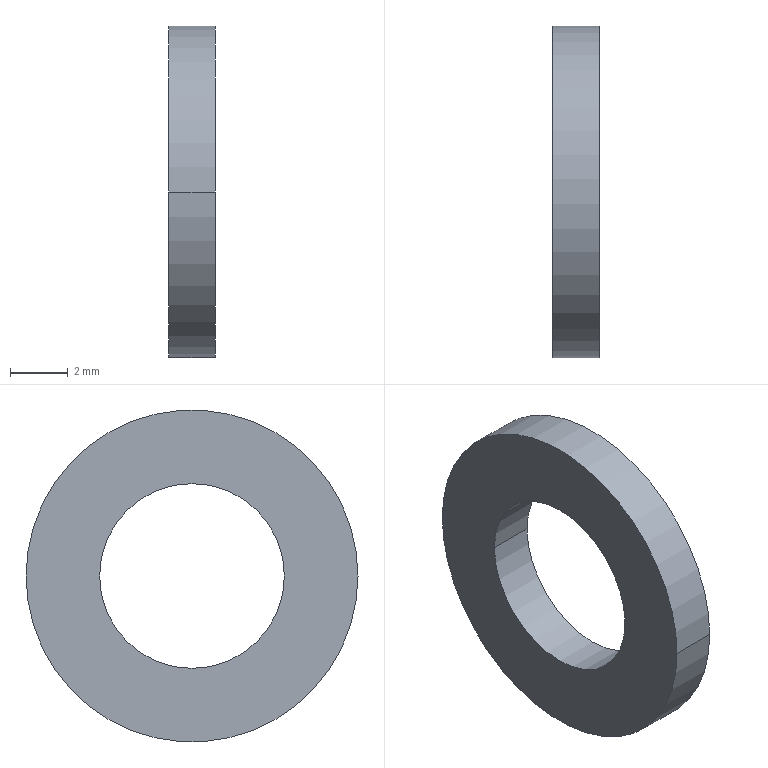Part | STEP file | KS B 1326 - 6x11.5 | 1 solid | 6 faces | box 1.6 x 11.5 x 11.5 mm | volume 114.718 mm3 | cylinder 4 | plane 2 | commonest cylinder face diameters 6.4 x2 11.5 x2
STEP:
#1=CARTESIAN_POINT('',(0.,0.,0.));
#2=DIRECTION('',(0.,0.,1.));
#3=DIRECTION('',(1.,0.,0.));
#4=AXIS2_PLACEMENT_3D('',#1,#2,#3);
#5=CARTESIAN_POINT('',(0.,-3.2,0.));
#6=VERTEX_POINT('',#5);
#7=CARTESIAN_POINT('',(1.6,-3.2,0.));
#8=VERTEX_POINT('',#7);
#9=CARTESIAN_POINT('',(0.,-3.2,0.));
#10=DIRECTION('',(1.,0.,0.));
#11=VECTOR('',#10,1.);
#12=LINE('',#9,#11);
#13=CARTESIAN_POINT('',(0.,0.,0.));
#14=DIRECTION('',(1.,0.,0.));
#15=DIRECTION('',(0.,-1.,0.));
#16=AXIS2_PLACEMENT_3D('',#13,#14,#15);
#17=CYLINDRICAL_SURFACE('',#16,3.2);
#18=CARTESIAN_POINT('',(6.283,0.));
#19=DIRECTION('',(0.,1.));
#20=VECTOR('',#19,1.);
#21=LINE('',#18,#20);
#22=(GEOMETRIC_REPRESENTATION_CONTEXT(2)PARAMETRIC_REPRESENTATION_CONTEXT()REPRESENTATION_CONTEXT('',''));
#23=DEFINITIONAL_REPRESENTATION('',(#21),#22);
#24=PCURVE('',#17,#23);
#25=CARTESIAN_POINT('',(0.,0.,0.));
#26=DIRECTION('',(1.,0.,0.));
#27=DIRECTION('',(0.,-1.,0.));
#28=AXIS2_PLACEMENT_3D('',#25,#26,#27);
#29=CYLINDRICAL_SURFACE('',#28,3.2);
#30=CARTESIAN_POINT('',(0.,0.));
#31=DIRECTION('',(0.,1.));
#32=VECTOR('',#31,1.);
#33=LINE('',#30,#32);
#34=(GEOMETRIC_REPRESENTATION_CONTEXT(2)PARAMETRIC_REPRESENTATION_CONTEXT()REPRESENTATION_CONTEXT('',''));
#35=DEFINITIONAL_REPRESENTATION('',(#33),#34);
#36=PCURVE('',#29,#35);
#37=SURFACE_CURVE('',#12,(#24,#36),.PCURVE_S1.);
#38=EDGE_CURVE('',#6,#8,#37,.T.);
#39=ORIENTED_EDGE('',*,*,#38,.T.);
#40=CARTESIAN_POINT('',(1.6,3.2,0.));
#41=VERTEX_POINT('',#40);
#42=CARTESIAN_POINT('',(1.6,0.,0.));
#43=DIRECTION('',(-1.,0.,0.));
#44=DIRECTION('',(0.,-1.,0.));
#45=AXIS2_PLACEMENT_3D('',#42,#43,#44);
#46=CIRCLE('',#45,3.2);
#47=CARTESIAN_POINT('',(6.283,1.6));
#48=DIRECTION('',(-1.,0.));
#49=VECTOR('',#48,1.);
#50=LINE('',#47,#49);
#51=(GEOMETRIC_REPRESENTATION_CONTEXT(2)PARAMETRIC_REPRESENTATION_CONTEXT()REPRESENTATION_CONTEXT('',''));
#52=DEFINITIONAL_REPRESENTATION('',(#50),#51);
#53=PCURVE('',#17,#52);
#54=CARTESIAN_POINT('',(1.6,0.,0.));
#55=DIRECTION('',(-1.,0.,0.));
#56=DIRECTION('',(0.,0.,1.));
#57=AXIS2_PLACEMENT_3D('',#54,#55,#56);
#58=PLANE('',#57);
#59=CARTESIAN_POINT('',(0.,0.));
#60=DIRECTION('',(0.,-1.));
#61=AXIS2_PLACEMENT_2D('',#59,#60);
#62=CIRCLE('',#61,3.2);
#63=(GEOMETRIC_REPRESENTATION_CONTEXT(2)PARAMETRIC_REPRESENTATION_CONTEXT()REPRESENTATION_CONTEXT('',''));
#64=DEFINITIONAL_REPRESENTATION('',(#62),#63);
#65=PCURVE('',#58,#64);
#66=SURFACE_CURVE('',#46,(#53,#65),.PCURVE_S1.);
#67=EDGE_CURVE('',#8,#41,#66,.T.);
#68=ORIENTED_EDGE('',*,*,#67,.T.);
#69=CARTESIAN_POINT('',(0.,3.2,0.));
#70=VERTEX_POINT('',#69);
#71=CARTESIAN_POINT('',(0.,3.2,0.));
#72=DIRECTION('',(1.,0.,0.));
#73=VECTOR('',#72,1.);
#74=LINE('',#71,#73);
#75=CARTESIAN_POINT('',(3.142,0.));
#76=DIRECTION('',(0.,1.));
#77=VECTOR('',#76,1.);
#78=LINE('',#75,#77);
#79=(GEOMETRIC_REPRESENTATION_CONTEXT(2)PARAMETRIC_REPRESENTATION_CONTEXT()REPRESENTATION_CONTEXT('',''));
#80=DEFINITIONAL_REPRESENTATION('',(#78),#79);
#81=PCURVE('',#17,#80);
#82=CARTESIAN_POINT('',(3.142,0.));
#83=DIRECTION('',(0.,1.));
#84=VECTOR('',#83,1.);
#85=LINE('',#82,#84);
#86=(GEOMETRIC_REPRESENTATION_CONTEXT(2)PARAMETRIC_REPRESENTATION_CONTEXT()REPRESENTATION_CONTEXT('',''));
#87=DEFINITIONAL_REPRESENTATION('',(#85),#86);
#88=PCURVE('',#29,#87);
#89=SURFACE_CURVE('',#74,(#81,#88),.PCURVE_S1.);
#90=EDGE_CURVE('',#70,#41,#89,.T.);
#91=ORIENTED_EDGE('',*,*,#90,.F.);
#92=CARTESIAN_POINT('',(0.,0.,0.));
#93=DIRECTION('',(1.,0.,0.));
#94=DIRECTION('',(0.,-1.,0.));
#95=AXIS2_PLACEMENT_3D('',#92,#93,#94);
#96=CIRCLE('',#95,3.2);
#97=CARTESIAN_POINT('',(0.,0.));
#98=DIRECTION('',(1.,0.));
#99=VECTOR('',#98,1.);
#100=LINE('',#97,#99);
#101=(GEOMETRIC_REPRESENTATION_CONTEXT(2)PARAMETRIC_REPRESENTATION_CONTEXT()REPRESENTATION_CONTEXT('',''));
#102=DEFINITIONAL_REPRESENTATION('',(#100),#101);
#103=PCURVE('',#17,#102);
#104=CARTESIAN_POINT('',(0.,0.,0.));
#105=DIRECTION('',(-1.,0.,0.));
#106=DIRECTION('',(0.,0.,1.));
#107=AXIS2_PLACEMENT_3D('',#104,#105,#106);
#108=PLANE('',#107);
#109=CARTESIAN_POINT('',(0.,-3.2));
#110=CARTESIAN_POINT('',(-5.543,-3.2));
#111=CARTESIAN_POINT('',(-2.771,1.6));
#112=CARTESIAN_POINT('',(0.,6.4));
#113=CARTESIAN_POINT('',(2.771,1.6));
#114=CARTESIAN_POINT('',(5.543,-3.2));
#115=CARTESIAN_POINT('',(0.,-3.2));
#116=(BOUNDED_CURVE()B_SPLINE_CURVE(2,(#109,#110,#111,#112,#113,#114,#115),.UNSPECIFIED.,.T.,.F.)B_SPLINE_CURVE_WITH_KNOTS((1,2,2,2,2,1),(-2.094,0.,2.094,4.189,6.283,8.378),.UNSPECIFIED.)CURVE()GEOMETRIC_REPRESENTATION_ITEM()RATIONAL_B_SPLINE_CURVE((1.,0.5,1.,0.5,1.,0.5,1.))REPRESENTATION_ITEM(''));
#117=(GEOMETRIC_REPRESENTATION_CONTEXT(2)PARAMETRIC_REPRESENTATION_CONTEXT()REPRESENTATION_CONTEXT('',''));
#118=DEFINITIONAL_REPRESENTATION('',(#116),#117);
#119=PCURVE('',#108,#118);
#120=SURFACE_CURVE('',#96,(#103,#119),.PCURVE_S1.);
#121=EDGE_CURVE('',#70,#6,#120,.T.);
#122=ORIENTED_EDGE('',*,*,#121,.T.);
#123=EDGE_LOOP('',(#39,#68,#91,#122));
#124=FACE_BOUND('',#123,.F.);
#125=ADVANCED_FACE('',(#124),#17,.F.);
#126=CARTESIAN_POINT('',(0.,5.75,0.));
#127=VERTEX_POINT('',#126);
#128=CARTESIAN_POINT('',(0.,-5.75,0.));
#129=VERTEX_POINT('',#128);
#130=CARTESIAN_POINT('',(0.,0.,0.));
#131=DIRECTION('',(-1.,0.,0.));
#132=DIRECTION('',(0.,-1.,0.));
#133=AXIS2_PLACEMENT_3D('',#130,#131,#132);
#134=CIRCLE('',#133,5.75);
#135=CARTESIAN_POINT('',(0.,0.,0.));
#136=DIRECTION('',(1.,0.,0.));
#137=DIRECTION('',(0.,-1.,0.));
#138=AXIS2_PLACEMENT_3D('',#135,#136,#137);
#139=CYLINDRICAL_SURFACE('',#138,5.75);
#140=CARTESIAN_POINT('',(6.283,0.));
#141=DIRECTION('',(-1.,0.));
#142=VECTOR('',#141,1.);
#143=LINE('',#140,#142);
#144=(GEOMETRIC_REPRESENTATION_CONTEXT(2)PARAMETRIC_REPRESENTATION_CONTEXT()REPRESENTATION_CONTEXT('',''));
#145=DEFINITIONAL_REPRESENTATION('',(#143),#144);
#146=PCURVE('',#139,#145);
#147=CARTESIAN_POINT('',(0.,0.));
#148=DIRECTION('',(0.,-1.));
#149=AXIS2_PLACEMENT_2D('',#147,#148);
#150=CIRCLE('',#149,5.75);
#151=(GEOMETRIC_REPRESENTATION_CONTEXT(2)PARAMETRIC_REPRESENTATION_CONTEXT()REPRESENTATION_CONTEXT('',''));
#152=DEFINITIONAL_REPRESENTATION('',(#150),#151);
#153=PCURVE('',#108,#152);
#154=SURFACE_CURVE('',#134,(#146,#153),.PCURVE_S1.);
#155=EDGE_CURVE('',#127,#129,#154,.T.);
#156=ORIENTED_EDGE('',*,*,#155,.F.);
#157=CARTESIAN_POINT('',(1.6,5.75,0.));
#158=VERTEX_POINT('',#157);
#159=CARTESIAN_POINT('',(0.,5.75,0.));
#160=DIRECTION('',(1.,0.,0.));
#161=VECTOR('',#160,1.);
#162=LINE('',#159,#161);
#163=CARTESIAN_POINT('',(3.142,0.));
#164=DIRECTION('',(0.,1.));
#165=VECTOR('',#164,1.);
#166=LINE('',#163,#165);
#167=(GEOMETRIC_REPRESENTATION_CONTEXT(2)PARAMETRIC_REPRESENTATION_CONTEXT()REPRESENTATION_CONTEXT('',''));
#168=DEFINITIONAL_REPRESENTATION('',(#166),#167);
#169=PCURVE('',#139,#168);
#170=CARTESIAN_POINT('',(0.,0.,0.));
#171=DIRECTION('',(1.,0.,0.));
#172=DIRECTION('',(0.,-1.,0.));
#173=AXIS2_PLACEMENT_3D('',#170,#171,#172);
#174=CYLINDRICAL_SURFACE('',#173,5.75);
#175=CARTESIAN_POINT('',(3.142,0.));
#176=DIRECTION('',(0.,1.));
#177=VECTOR('',#176,1.);
#178=LINE('',#175,#177);
#179=(GEOMETRIC_REPRESENTATION_CONTEXT(2)PARAMETRIC_REPRESENTATION_CONTEXT()REPRESENTATION_CONTEXT('',''));
#180=DEFINITIONAL_REPRESENTATION('',(#178),#179);
#181=PCURVE('',#174,#180);
#182=SURFACE_CURVE('',#162,(#169,#181),.PCURVE_S1.);
#183=EDGE_CURVE('',#127,#158,#182,.T.);
#184=ORIENTED_EDGE('',*,*,#183,.T.);
#185=CARTESIAN_POINT('',(1.6,-5.75,0.));
#186=VERTEX_POINT('',#185);
#187=CARTESIAN_POINT('',(1.6,0.,0.));
#188=DIRECTION('',(-1.,0.,0.));
#189=DIRECTION('',(0.,-1.,0.));
#190=AXIS2_PLACEMENT_3D('',#187,#188,#189);
#191=CIRCLE('',#190,5.75);
#192=CARTESIAN_POINT('',(6.283,1.6));
#193=DIRECTION('',(-1.,0.));
#194=VECTOR('',#193,1.);
#195=LINE('',#192,#194);
#196=(GEOMETRIC_REPRESENTATION_CONTEXT(2)PARAMETRIC_REPRESENTATION_CONTEXT()REPRESENTATION_CONTEXT('',''));
#197=DEFINITIONAL_REPRESENTATION('',(#195),#196);
#198=PCURVE('',#139,#197);
#199=CARTESIAN_POINT('',(0.,0.));
#200=DIRECTION('',(0.,-1.));
#201=AXIS2_PLACEMENT_2D('',#199,#200);
#202=CIRCLE('',#201,5.75);
#203=(GEOMETRIC_REPRESENTATION_CONTEXT(2)PARAMETRIC_REPRESENTATION_CONTEXT()REPRESENTATION_CONTEXT('',''));
#204=DEFINITIONAL_REPRESENTATION('',(#202),#203);
#205=PCURVE('',#58,#204);
#206=SURFACE_CURVE('',#191,(#198,#205),.PCURVE_S1.);
#207=EDGE_CURVE('',#158,#186,#206,.T.);
#208=ORIENTED_EDGE('',*,*,#207,.T.);
#209=CARTESIAN_POINT('',(0.,-5.75,0.));
#210=DIRECTION('',(1.,0.,0.));
#211=VECTOR('',#210,1.);
#212=LINE('',#209,#211);
#213=CARTESIAN_POINT('',(0.,0.));
#214=DIRECTION('',(0.,1.));
#215=VECTOR('',#214,1.);
#216=LINE('',#213,#215);
#217=(GEOMETRIC_REPRESENTATION_CONTEXT(2)PARAMETRIC_REPRESENTATION_CONTEXT()REPRESENTATION_CONTEXT('',''));
#218=DEFINITIONAL_REPRESENTATION('',(#216),#217);
#219=PCURVE('',#139,#218);
#220=CARTESIAN_POINT('',(6.283,0.));
#221=DIRECTION('',(0.,1.));
#222=VECTOR('',#221,1.);
#223=LINE('',#220,#222);
#224=(GEOMETRIC_REPRESENTATION_CONTEXT(2)PARAMETRIC_REPRESENTATION_CONTEXT()REPRESENTATION_CONTEXT('',''));
#225=DEFINITIONAL_REPRESENTATION('',(#223),#224);
#226=PCURVE('',#174,#225);
#227=SURFACE_CURVE('',#212,(#219,#226),.PCURVE_S1.);
#228=EDGE_CURVE('',#129,#186,#227,.T.);
#229=ORIENTED_EDGE('',*,*,#228,.F.);
#230=EDGE_LOOP('',(#156,#184,#208,#229));
#231=FACE_BOUND('',#230,.T.);
#232=ADVANCED_FACE('',(#231),#139,.T.);
#233=CARTESIAN_POINT('',(0.,0.,0.));
#234=DIRECTION('',(1.,0.,0.));
#235=DIRECTION('',(0.,-1.,0.));
#236=AXIS2_PLACEMENT_3D('',#233,#234,#235);
#237=CIRCLE('',#236,3.2);
#238=CARTESIAN_POINT('',(0.,-3.2));
#239=CARTESIAN_POINT('',(-5.543,-3.2));
#240=CARTESIAN_POINT('',(-2.771,1.6));
#241=CARTESIAN_POINT('',(0.,6.4));
#242=CARTESIAN_POINT('',(2.771,1.6));
#243=CARTESIAN_POINT('',(5.543,-3.2));
#244=CARTESIAN_POINT('',(0.,-3.2));
#245=(BOUNDED_CURVE()B_SPLINE_CURVE(2,(#238,#239,#240,#241,#242,#243,#244),.UNSPECIFIED.,.T.,.F.)B_SPLINE_CURVE_WITH_KNOTS((1,2,2,2,2,1),(-2.094,0.,2.094,4.189,6.283,8.378),.UNSPECIFIED.)CURVE()GEOMETRIC_REPRESENTATION_ITEM()RATIONAL_B_SPLINE_CURVE((1.,0.5,1.,0.5,1.,0.5,1.))REPRESENTATION_ITEM(''));
#246=(GEOMETRIC_REPRESENTATION_CONTEXT(2)PARAMETRIC_REPRESENTATION_CONTEXT()REPRESENTATION_CONTEXT('',''));
#247=DEFINITIONAL_REPRESENTATION('',(#245),#246);
#248=PCURVE('',#108,#247);
#249=CARTESIAN_POINT('',(0.,0.));
#250=DIRECTION('',(1.,0.));
#251=VECTOR('',#250,1.);
#252=LINE('',#249,#251);
#253=(GEOMETRIC_REPRESENTATION_CONTEXT(2)PARAMETRIC_REPRESENTATION_CONTEXT()REPRESENTATION_CONTEXT('',''));
#254=DEFINITIONAL_REPRESENTATION('',(#252),#253);
#255=PCURVE('',#29,#254);
#256=SURFACE_CURVE('',#237,(#248,#255),.PCURVE_S1.);
#257=EDGE_CURVE('',#6,#70,#256,.T.);
#258=ORIENTED_EDGE('',*,*,#257,.T.);
#259=ORIENTED_EDGE('',*,*,#121,.T.);
#260=EDGE_LOOP('',(#258,#259));
#261=FACE_BOUND('',#260,.T.);
#262=CARTESIAN_POINT('',(0.,0.,0.));
#263=DIRECTION('',(-1.,0.,0.));
#264=DIRECTION('',(0.,-1.,0.));
#265=AXIS2_PLACEMENT_3D('',#262,#263,#264);
#266=CIRCLE('',#265,5.75);
#267=CARTESIAN_POINT('',(0.,0.));
#268=DIRECTION('',(0.,-1.));
#269=AXIS2_PLACEMENT_2D('',#267,#268);
#270=CIRCLE('',#269,5.75);
#271=(GEOMETRIC_REPRESENTATION_CONTEXT(2)PARAMETRIC_REPRESENTATION_CONTEXT()REPRESENTATION_CONTEXT('',''));
#272=DEFINITIONAL_REPRESENTATION('',(#270),#271);
#273=PCURVE('',#108,#272);
#274=CARTESIAN_POINT('',(6.283,0.));
#275=DIRECTION('',(-1.,0.));
#276=VECTOR('',#275,1.);
#277=LINE('',#274,#276);
#278=(GEOMETRIC_REPRESENTATION_CONTEXT(2)PARAMETRIC_REPRESENTATION_CONTEXT()REPRESENTATION_CONTEXT('',''));
#279=DEFINITIONAL_REPRESENTATION('',(#277),#278);
#280=PCURVE('',#174,#279);
#281=SURFACE_CURVE('',#266,(#273,#280),.PCURVE_S1.);
#282=EDGE_CURVE('',#129,#127,#281,.T.);
#283=ORIENTED_EDGE('',*,*,#282,.T.);
#284=ORIENTED_EDGE('',*,*,#155,.T.);
#285=EDGE_LOOP('',(#283,#284));
#286=FACE_BOUND('',#285,.T.);
#287=ADVANCED_FACE('',(#261,#286),#108,.T.);
#288=ORIENTED_EDGE('',*,*,#67,.T.);
#289=CARTESIAN_POINT('',(1.6,0.,0.));
#290=DIRECTION('',(-1.,0.,0.));
#291=DIRECTION('',(0.,-1.,0.));
#292=AXIS2_PLACEMENT_3D('',#289,#290,#291);
#293=CIRCLE('',#292,3.2);
#294=CARTESIAN_POINT('',(0.,0.));
#295=DIRECTION('',(0.,-1.));
#296=AXIS2_PLACEMENT_2D('',#294,#295);
#297=CIRCLE('',#296,3.2);
#298=(GEOMETRIC_REPRESENTATION_CONTEXT(2)PARAMETRIC_REPRESENTATION_CONTEXT()REPRESENTATION_CONTEXT('',''));
#299=DEFINITIONAL_REPRESENTATION('',(#297),#298);
#300=PCURVE('',#58,#299);
#301=CARTESIAN_POINT('',(6.283,1.6));
#302=DIRECTION('',(-1.,0.));
#303=VECTOR('',#302,1.);
#304=LINE('',#301,#303);
#305=(GEOMETRIC_REPRESENTATION_CONTEXT(2)PARAMETRIC_REPRESENTATION_CONTEXT()REPRESENTATION_CONTEXT('',''));
#306=DEFINITIONAL_REPRESENTATION('',(#304),#305);
#307=PCURVE('',#29,#306);
#308=SURFACE_CURVE('',#293,(#300,#307),.PCURVE_S1.);
#309=EDGE_CURVE('',#41,#8,#308,.T.);
#310=ORIENTED_EDGE('',*,*,#309,.T.);
#311=EDGE_LOOP('',(#288,#310));
#312=FACE_BOUND('',#311,.T.);
#313=CARTESIAN_POINT('',(1.6,0.,0.));
#314=DIRECTION('',(-1.,0.,0.));
#315=DIRECTION('',(0.,-1.,0.));
#316=AXIS2_PLACEMENT_3D('',#313,#314,#315);
#317=CIRCLE('',#316,5.75);
#318=CARTESIAN_POINT('',(0.,0.));
#319=DIRECTION('',(0.,-1.));
#320=AXIS2_PLACEMENT_2D('',#318,#319);
#321=CIRCLE('',#320,5.75);
#322=(GEOMETRIC_REPRESENTATION_CONTEXT(2)PARAMETRIC_REPRESENTATION_CONTEXT()REPRESENTATION_CONTEXT('',''));
#323=DEFINITIONAL_REPRESENTATION('',(#321),#322);
#324=PCURVE('',#58,#323);
#325=CARTESIAN_POINT('',(6.283,1.6));
#326=DIRECTION('',(-1.,0.));
#327=VECTOR('',#326,1.);
#328=LINE('',#325,#327);
#329=(GEOMETRIC_REPRESENTATION_CONTEXT(2)PARAMETRIC_REPRESENTATION_CONTEXT()REPRESENTATION_CONTEXT('',''));
#330=DEFINITIONAL_REPRESENTATION('',(#328),#329);
#331=PCURVE('',#174,#330);
#332=SURFACE_CURVE('',#317,(#324,#331),.PCURVE_S1.);
#333=EDGE_CURVE('',#186,#158,#332,.T.);
#334=ORIENTED_EDGE('',*,*,#333,.F.);
#335=ORIENTED_EDGE('',*,*,#207,.F.);
#336=EDGE_LOOP('',(#334,#335));
#337=FACE_BOUND('',#336,.T.);
#338=ADVANCED_FACE('',(#312,#337),#58,.F.);
#339=ORIENTED_EDGE('',*,*,#183,.F.);
#340=ORIENTED_EDGE('',*,*,#282,.F.);
#341=ORIENTED_EDGE('',*,*,#228,.T.);
#342=ORIENTED_EDGE('',*,*,#333,.T.);
#343=EDGE_LOOP('',(#339,#340,#341,#342));
#344=FACE_BOUND('',#343,.T.);
#345=ADVANCED_FACE('',(#344),#174,.T.);
#346=ORIENTED_EDGE('',*,*,#309,.T.);
#347=ORIENTED_EDGE('',*,*,#38,.F.);
#348=ORIENTED_EDGE('',*,*,#257,.T.);
#349=ORIENTED_EDGE('',*,*,#90,.T.);
#350=EDGE_LOOP('',(#346,#347,#348,#349));
#351=FACE_BOUND('',#350,.F.);
#352=ADVANCED_FACE('',(#351),#29,.F.);
#353=CLOSED_SHELL('',(#125,#232,#287,#338,#345,#352));
#354=MANIFOLD_SOLID_BREP('',#353);
#355=(LENGTH_UNIT()NAMED_UNIT(*)SI_UNIT(.MILLI.,.METRE.));
#356=UNCERTAINTY_MEASURE_WITH_UNIT(LENGTH_MEASURE(0.0000001),#355,'','');
#357=(NAMED_UNIT(*)PLANE_ANGLE_UNIT()SI_UNIT($,.RADIAN.));
#358=(NAMED_UNIT(*)SI_UNIT($,.STERADIAN.)SOLID_ANGLE_UNIT());
#359=(GEOMETRIC_REPRESENTATION_CONTEXT(3)GLOBAL_UNCERTAINTY_ASSIGNED_CONTEXT((#356))GLOBAL_UNIT_ASSIGNED_CONTEXT((#355,#357,#358))REPRESENTATION_CONTEXT('',''));
#360=ADVANCED_BREP_SHAPE_REPRESENTATION('',(#4,#354),#359);